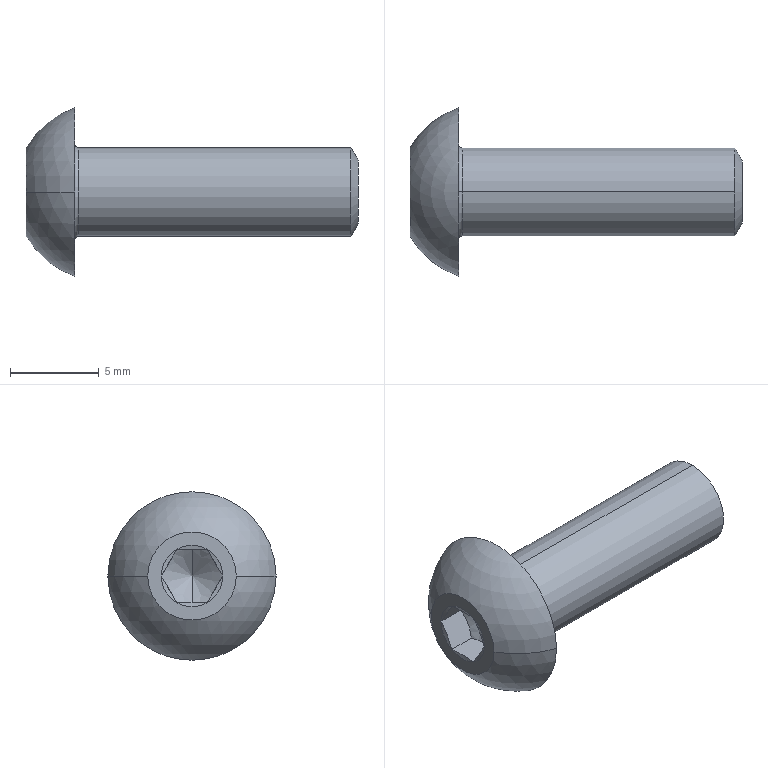Part | SolidWorks | features RevCut 2, Revolution 2, Cut 1, LPattern 1, RefAxis 1 | 1 solid | 25 faces | box 18.75 x 9.5 x 9.5 mm | volume 431.838 mm3 | cone 10 | plane 9 | torus 2 | sphere 2 | cylinder 2 | commonest cylinder face diameters 5 x2
STEP:
#1=CARTESIAN_POINT('',(0.,0.,1.807));
#2=VERTEX_POINT('',#1);
#3=CARTESIAN_POINT('',(0.,0.,-1.807));
#4=VERTEX_POINT('',#3);
#5=CARTESIAN_POINT('',(0.,0.,0.));
#6=DIRECTION('',(-1.,0.,0.));
#7=DIRECTION('',(0.,0.,1.));
#8=AXIS2_PLACEMENT_3D('',#5,#6,#7);
#9=CIRCLE('',#8,1.807);
#10=EDGE_CURVE('',#2,#4,#9,.T.);
#11=ORIENTED_EDGE('',*,*,#10,.T.);
#12=CARTESIAN_POINT('',(-0.4,0.,-2.5));
#13=VERTEX_POINT('',#12);
#14=CARTESIAN_POINT('',(-0.4,0.,-2.5));
#15=DIRECTION('',(-0.5,0.,-0.866));
#16=VECTOR('',#15,1000.);
#17=LINE('',#14,#16);
#18=EDGE_CURVE('',#4,#13,#17,.T.);
#19=ORIENTED_EDGE('',*,*,#18,.T.);
#20=CARTESIAN_POINT('',(-0.4,0.,2.5));
#21=VERTEX_POINT('',#20);
#22=CARTESIAN_POINT('',(-0.4,0.,0.));
#23=DIRECTION('',(-1.,0.,0.));
#24=DIRECTION('',(0.,0.,1.));
#25=AXIS2_PLACEMENT_3D('',#22,#23,#24);
#26=CIRCLE('',#25,2.5);
#27=EDGE_CURVE('',#21,#13,#26,.T.);
#28=ORIENTED_EDGE('',*,*,#27,.F.);
#29=CARTESIAN_POINT('',(-0.4,0.,2.5));
#30=DIRECTION('',(-0.5,0.,0.866));
#31=VECTOR('',#30,1000.);
#32=LINE('',#29,#31);
#33=EDGE_CURVE('',#2,#21,#32,.T.);
#34=ORIENTED_EDGE('',*,*,#33,.F.);
#35=EDGE_LOOP('',(#11,#19,#28,#34));
#36=FACE_OUTER_BOUND('',#35,.T.);
#37=CARTESIAN_POINT('',(-0.4,0.,0.));
#38=DIRECTION('',(-1.,0.,0.));
#39=DIRECTION('',(0.,0.,1.));
#40=AXIS2_PLACEMENT_3D('',#37,#38,#39);
#41=CONICAL_SURFACE('',#40,2.5,1.047);
#42=ADVANCED_FACE('',(#36),#41,.T.);
#43=CARTESIAN_POINT('',(-16.,0.,0.));
#44=VERTEX_POINT('',#43);
#45=CARTESIAN_POINT('',(-17.031,0.,1.5));
#46=VERTEX_POINT('',#45);
#47=CARTESIAN_POINT('',(-17.19,0.,1.732));
#48=DIRECTION('',(-0.5663,0.,0.8242));
#49=VECTOR('',#48,1000.);
#50=LINE('',#47,#49);
#51=EDGE_CURVE('',#44,#46,#50,.T.);
#52=ORIENTED_EDGE('',*,*,#51,.F.);
#53=CARTESIAN_POINT('',(-17.031,0.,-1.5));
#54=VERTEX_POINT('',#53);
#55=CARTESIAN_POINT('',(-17.19,0.,-1.732));
#56=DIRECTION('',(-0.5663,0.,-0.8242));
#57=VECTOR('',#56,1000.);
#58=LINE('',#55,#57);
#59=EDGE_CURVE('',#44,#54,#58,.T.);
#60=ORIENTED_EDGE('',*,*,#59,.T.);
#61=CARTESIAN_POINT('',(-17.19,-0.866,-1.5));
#62=VERTEX_POINT('',#61);
#63=CARTESIAN_POINT('',(-17.031,0.,-1.5));
#64=CARTESIAN_POINT('',(-17.031,-0.147,-1.5));
#65=CARTESIAN_POINT('',(-17.046,-0.2929,-1.5));
#66=CARTESIAN_POINT('',(-17.101,-0.5828,-1.5));
#67=CARTESIAN_POINT('',(-17.142,-0.7267,-1.5));
#68=CARTESIAN_POINT('',(-17.19,-0.866,-1.5));
#69=B_SPLINE_CURVE_WITH_KNOTS('',3,(#63,#64,#65,#66,#67,#68),.UNSPECIFIED.,.F.,.F.,(4,2,4),(0.005367,0.005808,0.006249),.UNSPECIFIED.);
#70=EDGE_CURVE('',#54,#62,#69,.T.);
#71=ORIENTED_EDGE('',*,*,#70,.T.);
#72=CARTESIAN_POINT('',(-17.19,-1.732,0.));
#73=VERTEX_POINT('',#72);
#74=CARTESIAN_POINT('',(-17.19,-0.866,-1.5));
#75=CARTESIAN_POINT('',(-17.094,-1.006,-1.257));
#76=CARTESIAN_POINT('',(-17.031,-1.149,-1.009));
#77=CARTESIAN_POINT('',(-17.03,-1.372,-0.6244));
#78=CARTESIAN_POINT('',(-17.046,-1.446,-0.4956));
#79=CARTESIAN_POINT('',(-17.102,-1.591,-0.2449));
#80=CARTESIAN_POINT('',(-17.142,-1.662,-0.1218));
#81=CARTESIAN_POINT('',(-17.19,-1.732,0.));
#82=B_SPLINE_CURVE_WITH_KNOTS('',3,(#74,#75,#76,#77,#78,#79,#80,#81),.UNSPECIFIED.,.F.,.F.,(4,2,2,4),(0.000000241,0.0008776,0.001316,0.001755),.UNSPECIFIED.);
#83=EDGE_CURVE('',#62,#73,#82,.T.);
#84=ORIENTED_EDGE('',*,*,#83,.T.);
#85=CARTESIAN_POINT('',(-17.19,-0.866,1.5));
#86=VERTEX_POINT('',#85);
#87=CARTESIAN_POINT('',(-17.19,-1.732,0.));
#88=CARTESIAN_POINT('',(-17.094,-1.592,0.2429));
#89=CARTESIAN_POINT('',(-17.031,-1.449,0.4906));
#90=CARTESIAN_POINT('',(-17.03,-1.227,0.8756));
#91=CARTESIAN_POINT('',(-17.046,-1.152,1.004));
#92=CARTESIAN_POINT('',(-17.102,-1.007,1.255));
#93=CARTESIAN_POINT('',(-17.142,-0.9363,1.378));
#94=CARTESIAN_POINT('',(-17.19,-0.866,1.5));
#95=B_SPLINE_CURVE_WITH_KNOTS('',3,(#87,#88,#89,#90,#91,#92,#93,#94),.UNSPECIFIED.,.F.,.F.,(4,2,2,4),(0.000000241,0.0008776,0.001316,0.001755),.UNSPECIFIED.);
#96=EDGE_CURVE('',#73,#86,#95,.T.);
#97=ORIENTED_EDGE('',*,*,#96,.T.);
#98=CARTESIAN_POINT('',(-17.19,-0.866,1.5));
#99=CARTESIAN_POINT('',(-17.142,-0.7267,1.5));
#100=CARTESIAN_POINT('',(-17.101,-0.5828,1.5));
#101=CARTESIAN_POINT('',(-17.046,-0.2929,1.5));
#102=CARTESIAN_POINT('',(-17.031,-0.147,1.5));
#103=CARTESIAN_POINT('',(-17.031,0.,1.5));
#104=B_SPLINE_CURVE_WITH_KNOTS('',3,(#98,#99,#100,#101,#102,#103),.UNSPECIFIED.,.F.,.F.,(4,2,4),(0.001244,0.001684,0.002125),.UNSPECIFIED.);
#105=EDGE_CURVE('',#86,#46,#104,.T.);
#106=ORIENTED_EDGE('',*,*,#105,.T.);
#107=EDGE_LOOP('',(#52,#60,#71,#84,#97,#106));
#108=FACE_OUTER_BOUND('',#107,.T.);
#109=CARTESIAN_POINT('',(-17.19,0.,0.));
#110=DIRECTION('',(-1.,0.,0.));
#111=DIRECTION('',(0.,0.,1.));
#112=AXIS2_PLACEMENT_3D('',#109,#110,#111);
#113=CONICAL_SURFACE('',#112,1.732,0.9688);
#114=ADVANCED_FACE('',(#108),#113,.F.);
#115=CARTESIAN_POINT('',(-16.,0.,-2.7));
#116=VERTEX_POINT('',#115);
#117=CARTESIAN_POINT('',(-16.,0.,2.7));
#118=VERTEX_POINT('',#117);
#119=CARTESIAN_POINT('',(-16.,0.,0.));
#120=DIRECTION('',(-1.,0.,0.));
#121=DIRECTION('',(0.,0.,1.));
#122=AXIS2_PLACEMENT_3D('',#119,#120,#121);
#123=CIRCLE('',#122,2.7);
#124=EDGE_CURVE('',#116,#118,#123,.T.);
#125=ORIENTED_EDGE('',*,*,#124,.F.);
#126=CARTESIAN_POINT('',(-15.8,0.,-2.5));
#127=VERTEX_POINT('',#126);
#128=CARTESIAN_POINT('',(-15.8,0.,-2.7));
#129=DIRECTION('',(0.,1.,0.));
#130=DIRECTION('',(0.,0.,1.));
#131=AXIS2_PLACEMENT_3D('',#128,#129,#130);
#132=CIRCLE('',#131,0.2);
#133=EDGE_CURVE('',#116,#127,#132,.T.);
#134=ORIENTED_EDGE('',*,*,#133,.T.);
#135=CARTESIAN_POINT('',(-15.8,0.,2.5));
#136=VERTEX_POINT('',#135);
#137=CARTESIAN_POINT('',(-15.8,0.,0.));
#138=DIRECTION('',(-1.,0.,0.));
#139=DIRECTION('',(0.,0.,1.));
#140=AXIS2_PLACEMENT_3D('',#137,#138,#139);
#141=CIRCLE('',#140,2.5);
#142=EDGE_CURVE('',#127,#136,#141,.T.);
#143=ORIENTED_EDGE('',*,*,#142,.T.);
#144=CARTESIAN_POINT('',(-15.8,0.,2.7));
#145=DIRECTION('',(0.,-1.,0.));
#146=DIRECTION('',(0.,0.,-1.));
#147=AXIS2_PLACEMENT_3D('',#144,#145,#146);
#148=CIRCLE('',#147,0.2);
#149=EDGE_CURVE('',#118,#136,#148,.T.);
#150=ORIENTED_EDGE('',*,*,#149,.F.);
#151=EDGE_LOOP('',(#125,#134,#143,#150));
#152=FACE_OUTER_BOUND('',#151,.T.);
#153=CARTESIAN_POINT('',(-15.8,0.,0.));
#154=DIRECTION('',(-1.,0.,0.));
#155=DIRECTION('',(0.,0.,1.));
#156=AXIS2_PLACEMENT_3D('',#153,#154,#155);
#157=TOROIDAL_SURFACE('',#156,2.7,0.2);
#158=ADVANCED_FACE('',(#152),#157,.F.);
#159=CARTESIAN_POINT('',(-16.,4.75,0.));
#160=VERTEX_POINT('',#159);
#161=CARTESIAN_POINT('',(-16.,-4.75,0.));
#162=VERTEX_POINT('',#161);
#163=CARTESIAN_POINT('',(-16.,0.,0.));
#164=DIRECTION('',(-1.,0.,0.));
#165=DIRECTION('',(0.,0.,1.));
#166=AXIS2_PLACEMENT_3D('',#163,#164,#165);
#167=CIRCLE('',#166,4.75);
#168=EDGE_CURVE('',#160,#162,#167,.T.);
#169=ORIENTED_EDGE('',*,*,#168,.T.);
#170=CARTESIAN_POINT('',(-18.75,-2.5,0.));
#171=VERTEX_POINT('',#170);
#172=CARTESIAN_POINT('',(-14.409,0.,0.));
#173=DIRECTION('',(0.,0.,-1.));
#174=DIRECTION('',(0.,1.,0.));
#175=AXIS2_PLACEMENT_3D('',#172,#173,#174);
#176=CIRCLE('',#175,5.009);
#177=EDGE_CURVE('',#162,#171,#176,.T.);
#178=ORIENTED_EDGE('',*,*,#177,.T.);
#179=CARTESIAN_POINT('',(-18.75,2.5,0.));
#180=VERTEX_POINT('',#179);
#181=CARTESIAN_POINT('',(-18.75,0.,0.));
#182=DIRECTION('',(-1.,0.,0.));
#183=DIRECTION('',(0.,0.,1.));
#184=AXIS2_PLACEMENT_3D('',#181,#182,#183);
#185=CIRCLE('',#184,2.5);
#186=EDGE_CURVE('',#180,#171,#185,.T.);
#187=ORIENTED_EDGE('',*,*,#186,.F.);
#188=CARTESIAN_POINT('',(-14.409,0.,0.));
#189=DIRECTION('',(0.,0.,1.));
#190=DIRECTION('',(1.,0.,0.));
#191=AXIS2_PLACEMENT_3D('',#188,#189,#190);
#192=CIRCLE('',#191,5.009);
#193=EDGE_CURVE('',#160,#180,#192,.T.);
#194=ORIENTED_EDGE('',*,*,#193,.F.);
#195=EDGE_LOOP('',(#169,#178,#187,#194));
#196=FACE_OUTER_BOUND('',#195,.T.);
#197=CARTESIAN_POINT('',(-14.409,0.,0.));
#198=DIRECTION('',(0.,0.,-1.));
#199=DIRECTION('',(0.,1.,0.));
#200=AXIS2_PLACEMENT_3D('',#197,#198,#199);
#201=SPHERICAL_SURFACE('',#200,5.009);
#202=ADVANCED_FACE('',(#196),#201,.T.);
#203=ORIENTED_EDGE('',*,*,#27,.T.);
#204=CARTESIAN_POINT('',(-18.75,0.,-2.5));
#205=DIRECTION('',(-1.,0.,0.));
#206=VECTOR('',#205,1000.);
#207=LINE('',#204,#206);
#208=EDGE_CURVE('',#13,#127,#207,.T.);
#209=ORIENTED_EDGE('',*,*,#208,.T.);
#210=CARTESIAN_POINT('',(-15.8,0.,0.));
#211=DIRECTION('',(-1.,0.,0.));
#212=DIRECTION('',(0.,0.,1.));
#213=AXIS2_PLACEMENT_3D('',#210,#211,#212);
#214=CIRCLE('',#213,2.5);
#215=EDGE_CURVE('',#136,#127,#214,.T.);
#216=ORIENTED_EDGE('',*,*,#215,.F.);
#217=CARTESIAN_POINT('',(-18.75,0.,2.5));
#218=DIRECTION('',(-1.,0.,0.));
#219=VECTOR('',#218,1000.);
#220=LINE('',#217,#219);
#221=EDGE_CURVE('',#21,#136,#220,.T.);
#222=ORIENTED_EDGE('',*,*,#221,.F.);
#223=EDGE_LOOP('',(#203,#209,#216,#222));
#224=FACE_OUTER_BOUND('',#223,.T.);
#225=CARTESIAN_POINT('',(-18.75,0.,0.));
#226=DIRECTION('',(-1.,0.,0.));
#227=DIRECTION('',(0.,0.,1.));
#228=AXIS2_PLACEMENT_3D('',#225,#226,#227);
#229=CYLINDRICAL_SURFACE('',#228,2.5);
#230=ADVANCED_FACE('',(#224),#229,.T.);
#231=ORIENTED_EDGE('',*,*,#208,.F.);
#232=CARTESIAN_POINT('',(-0.4,0.,0.));
#233=DIRECTION('',(-1.,0.,0.));
#234=DIRECTION('',(0.,0.,1.));
#235=AXIS2_PLACEMENT_3D('',#232,#233,#234);
#236=CIRCLE('',#235,2.5);
#237=EDGE_CURVE('',#13,#21,#236,.T.);
#238=ORIENTED_EDGE('',*,*,#237,.T.);
#239=ORIENTED_EDGE('',*,*,#221,.T.);
#240=ORIENTED_EDGE('',*,*,#142,.F.);
#241=EDGE_LOOP('',(#231,#238,#239,#240));
#242=FACE_OUTER_BOUND('',#241,.T.);
#243=CARTESIAN_POINT('',(-18.75,0.,0.));
#244=DIRECTION('',(-1.,0.,0.));
#245=DIRECTION('',(0.,0.,1.));
#246=AXIS2_PLACEMENT_3D('',#243,#244,#245);
#247=CYLINDRICAL_SURFACE('',#246,2.5);
#248=ADVANCED_FACE('',(#242),#247,.T.);
#249=ORIENTED_EDGE('',*,*,#186,.T.);
#250=CARTESIAN_POINT('',(-18.75,0.,0.));
#251=DIRECTION('',(-1.,0.,0.));
#252=DIRECTION('',(0.,0.,1.));
#253=AXIS2_PLACEMENT_3D('',#250,#251,#252);
#254=CIRCLE('',#253,2.5);
#255=EDGE_CURVE('',#171,#180,#254,.T.);
#256=ORIENTED_EDGE('',*,*,#255,.T.);
#257=EDGE_LOOP('',(#249,#256));
#258=FACE_OUTER_BOUND('',#257,.T.);
#259=CARTESIAN_POINT('',(-18.75,-0.866,-1.5));
#260=VERTEX_POINT('',#259);
#261=CARTESIAN_POINT('',(-18.75,-1.732,0.));
#262=VERTEX_POINT('',#261);
#263=CARTESIAN_POINT('',(-18.75,0.,0.));
#264=DIRECTION('',(-1.,0.,0.));
#265=DIRECTION('',(0.,0.,-1.));
#266=AXIS2_PLACEMENT_3D('',#263,#264,#265);
#267=CIRCLE('',#266,1.732);
#268=EDGE_CURVE('',#260,#262,#267,.T.);
#269=ORIENTED_EDGE('',*,*,#268,.F.);
#270=CARTESIAN_POINT('',(-18.75,0.866,-1.5));
#271=VERTEX_POINT('',#270);
#272=CARTESIAN_POINT('',(-18.75,0.,0.));
#273=DIRECTION('',(-1.,0.,0.));
#274=DIRECTION('',(0.,0.,-1.));
#275=AXIS2_PLACEMENT_3D('',#272,#273,#274);
#276=CIRCLE('',#275,1.732);
#277=EDGE_CURVE('',#271,#260,#276,.T.);
#278=ORIENTED_EDGE('',*,*,#277,.F.);
#279=CARTESIAN_POINT('',(-18.75,1.732,0.));
#280=VERTEX_POINT('',#279);
#281=CARTESIAN_POINT('',(-18.75,0.,0.));
#282=DIRECTION('',(-1.,0.,0.));
#283=DIRECTION('',(0.,0.,-1.));
#284=AXIS2_PLACEMENT_3D('',#281,#282,#283);
#285=CIRCLE('',#284,1.732);
#286=EDGE_CURVE('',#280,#271,#285,.T.);
#287=ORIENTED_EDGE('',*,*,#286,.F.);
#288=CARTESIAN_POINT('',(-18.75,0.866,1.5));
#289=VERTEX_POINT('',#288);
#290=CARTESIAN_POINT('',(-18.75,0.,0.));
#291=DIRECTION('',(-1.,0.,0.));
#292=DIRECTION('',(0.,0.,-1.));
#293=AXIS2_PLACEMENT_3D('',#290,#291,#292);
#294=CIRCLE('',#293,1.732);
#295=EDGE_CURVE('',#289,#280,#294,.T.);
#296=ORIENTED_EDGE('',*,*,#295,.F.);
#297=CARTESIAN_POINT('',(-18.75,-0.866,1.5));
#298=VERTEX_POINT('',#297);
#299=CARTESIAN_POINT('',(-18.75,0.,0.));
#300=DIRECTION('',(-1.,0.,0.));
#301=DIRECTION('',(0.,0.,-1.));
#302=AXIS2_PLACEMENT_3D('',#299,#300,#301);
#303=CIRCLE('',#302,1.732);
#304=EDGE_CURVE('',#298,#289,#303,.T.);
#305=ORIENTED_EDGE('',*,*,#304,.F.);
#306=CARTESIAN_POINT('',(-18.75,0.,0.));
#307=DIRECTION('',(-1.,0.,0.));
#308=DIRECTION('',(0.,-1.,0.));
#309=AXIS2_PLACEMENT_3D('',#306,#307,#308);
#310=CIRCLE('',#309,1.732);
#311=EDGE_CURVE('',#262,#298,#310,.T.);
#312=ORIENTED_EDGE('',*,*,#311,.F.);
#313=EDGE_LOOP('',(#269,#278,#287,#296,#305,#312));
#314=FACE_BOUND('',#313,.T.);
#315=CARTESIAN_POINT('',(-18.75,0.,0.));
#316=DIRECTION('',(1.,0.,0.));
#317=DIRECTION('',(0.,0.,-1.));
#318=AXIS2_PLACEMENT_3D('',#315,#316,#317);
#319=PLANE('',#318);
#320=ADVANCED_FACE('',(#258,#314),#319,.F.);
#321=ORIENTED_EDGE('',*,*,#177,.F.);
#322=CARTESIAN_POINT('',(-16.,0.,0.));
#323=DIRECTION('',(-1.,0.,0.));
#324=DIRECTION('',(0.,0.,1.));
#325=AXIS2_PLACEMENT_3D('',#322,#323,#324);
#326=CIRCLE('',#325,4.75);
#327=EDGE_CURVE('',#162,#160,#326,.T.);
#328=ORIENTED_EDGE('',*,*,#327,.T.);
#329=ORIENTED_EDGE('',*,*,#193,.T.);
#330=ORIENTED_EDGE('',*,*,#255,.F.);
#331=EDGE_LOOP('',(#321,#328,#329,#330));
#332=FACE_OUTER_BOUND('',#331,.T.);
#333=CARTESIAN_POINT('',(-14.409,0.,0.));
#334=DIRECTION('',(0.,0.,-1.));
#335=DIRECTION('',(0.,1.,0.));
#336=AXIS2_PLACEMENT_3D('',#333,#334,#335);
#337=SPHERICAL_SURFACE('',#336,5.009);
#338=ADVANCED_FACE('',(#332),#337,.T.);
#339=ORIENTED_EDGE('',*,*,#168,.F.);
#340=ORIENTED_EDGE('',*,*,#327,.F.);
#341=EDGE_LOOP('',(#339,#340));
#342=FACE_OUTER_BOUND('',#341,.T.);
#343=CARTESIAN_POINT('',(-16.,0.,0.));
#344=DIRECTION('',(-1.,0.,0.));
#345=DIRECTION('',(0.,0.,1.));
#346=AXIS2_PLACEMENT_3D('',#343,#344,#345);
#347=CIRCLE('',#346,2.7);
#348=EDGE_CURVE('',#118,#116,#347,.T.);
#349=ORIENTED_EDGE('',*,*,#348,.T.);
#350=ORIENTED_EDGE('',*,*,#124,.T.);
#351=EDGE_LOOP('',(#349,#350));
#352=FACE_BOUND('',#351,.T.);
#353=CARTESIAN_POINT('',(-16.,2.7,0.));
#354=DIRECTION('',(-1.,0.,0.));
#355=DIRECTION('',(0.,0.,1.));
#356=AXIS2_PLACEMENT_3D('',#353,#354,#355);
#357=PLANE('',#356);
#358=ADVANCED_FACE('',(#342,#352),#357,.F.);
#359=ORIENTED_EDGE('',*,*,#133,.F.);
#360=ORIENTED_EDGE('',*,*,#348,.F.);
#361=ORIENTED_EDGE('',*,*,#149,.T.);
#362=ORIENTED_EDGE('',*,*,#215,.T.);
#363=EDGE_LOOP('',(#359,#360,#361,#362));
#364=FACE_OUTER_BOUND('',#363,.T.);
#365=CARTESIAN_POINT('',(-15.8,0.,0.));
#366=DIRECTION('',(-1.,0.,0.));
#367=DIRECTION('',(0.,0.,1.));
#368=AXIS2_PLACEMENT_3D('',#365,#366,#367);
#369=TOROIDAL_SURFACE('',#368,2.7,0.2);
#370=ADVANCED_FACE('',(#364),#369,.F.);
#371=CARTESIAN_POINT('',(-18.75,-0.866,-1.5));
#372=CARTESIAN_POINT('',(-18.713,-0.5778,-1.5));
#373=CARTESIAN_POINT('',(-18.691,-0.2874,-1.5));
#374=CARTESIAN_POINT('',(-18.691,0.2902,-1.5));
#375=CARTESIAN_POINT('',(-18.713,0.5783,-1.5));
#376=CARTESIAN_POINT('',(-18.75,0.866,-1.5));
#377=B_SPLINE_CURVE_WITH_KNOTS('',3,(#371,#372,#373,#374,#375,#376),.UNSPECIFIED.,.F.,.F.,(4,2,4),(0.001419,0.00229,0.003161),.UNSPECIFIED.);
#378=EDGE_CURVE('',#260,#271,#377,.T.);
#379=ORIENTED_EDGE('',*,*,#378,.T.);
#380=ORIENTED_EDGE('',*,*,#277,.T.);
#381=EDGE_LOOP('',(#379,#380));
#382=FACE_OUTER_BOUND('',#381,.T.);
#383=CARTESIAN_POINT('',(-1018.31,0.,0.));
#384=DIRECTION('',(-1.,0.,0.));
#385=DIRECTION('',(0.,-1.,0.));
#386=AXIS2_PLACEMENT_3D('',#383,#384,#385);
#387=CONICAL_SURFACE('',#386,3936.479,1.322);
#388=ADVANCED_FACE('',(#382),#387,.F.);
#389=CARTESIAN_POINT('',(-18.75,0.866,-1.5));
#390=CARTESIAN_POINT('',(-18.713,1.01,-1.25));
#391=CARTESIAN_POINT('',(-18.669,1.299,-0.75));
#392=CARTESIAN_POINT('',(-18.713,1.588,-0.25));
#393=CARTESIAN_POINT('',(-18.75,1.732,0.));
#394=B_SPLINE_CURVE_WITH_KNOTS('',3,(#389,#390,#391,#392,#393),.UNSPECIFIED.,.F.,.F.,(4,1,4),(0.000000231,0.0008663,0.001732),.UNSPECIFIED.);
#395=EDGE_CURVE('',#271,#280,#394,.T.);
#396=ORIENTED_EDGE('',*,*,#395,.T.);
#397=ORIENTED_EDGE('',*,*,#286,.T.);
#398=EDGE_LOOP('',(#396,#397));
#399=FACE_OUTER_BOUND('',#398,.T.);
#400=CARTESIAN_POINT('',(-1018.31,0.,0.));
#401=DIRECTION('',(-1.,0.,0.));
#402=DIRECTION('',(0.,-1.,0.));
#403=AXIS2_PLACEMENT_3D('',#400,#401,#402);
#404=CONICAL_SURFACE('',#403,3936.479,1.322);
#405=ADVANCED_FACE('',(#399),#404,.F.);
#406=CARTESIAN_POINT('',(-18.75,1.732,0.));
#407=CARTESIAN_POINT('',(-18.713,1.588,0.25));
#408=CARTESIAN_POINT('',(-18.669,1.299,0.75));
#409=CARTESIAN_POINT('',(-18.713,1.01,1.25));
#410=CARTESIAN_POINT('',(-18.75,0.866,1.5));
#411=B_SPLINE_CURVE_WITH_KNOTS('',3,(#406,#407,#408,#409,#410),.UNSPECIFIED.,.F.,.F.,(4,1,4),(0.000000231,0.0008663,0.001732),.UNSPECIFIED.);
#412=EDGE_CURVE('',#280,#289,#411,.T.);
#413=ORIENTED_EDGE('',*,*,#412,.T.);
#414=ORIENTED_EDGE('',*,*,#295,.T.);
#415=EDGE_LOOP('',(#413,#414));
#416=FACE_OUTER_BOUND('',#415,.T.);
#417=CARTESIAN_POINT('',(-1018.31,0.,0.));
#418=DIRECTION('',(-1.,0.,0.));
#419=DIRECTION('',(0.,-1.,0.));
#420=AXIS2_PLACEMENT_3D('',#417,#418,#419);
#421=CONICAL_SURFACE('',#420,3936.479,1.322);
#422=ADVANCED_FACE('',(#416),#421,.F.);
#423=CARTESIAN_POINT('',(-18.75,0.866,1.5));
#424=CARTESIAN_POINT('',(-18.713,0.5783,1.5));
#425=CARTESIAN_POINT('',(-18.691,0.2902,1.5));
#426=CARTESIAN_POINT('',(-18.691,-0.2874,1.5));
#427=CARTESIAN_POINT('',(-18.713,-0.5778,1.5));
#428=CARTESIAN_POINT('',(-18.75,-0.866,1.5));
#429=B_SPLINE_CURVE_WITH_KNOTS('',3,(#423,#424,#425,#426,#427,#428),.UNSPECIFIED.,.F.,.F.,(4,2,4),(0.003564,0.004433,0.005303),.UNSPECIFIED.);
#430=EDGE_CURVE('',#289,#298,#429,.T.);
#431=ORIENTED_EDGE('',*,*,#430,.T.);
#432=ORIENTED_EDGE('',*,*,#304,.T.);
#433=EDGE_LOOP('',(#431,#432));
#434=FACE_OUTER_BOUND('',#433,.T.);
#435=CARTESIAN_POINT('',(-1018.31,0.,0.));
#436=DIRECTION('',(-1.,0.,0.));
#437=DIRECTION('',(0.,-1.,0.));
#438=AXIS2_PLACEMENT_3D('',#435,#436,#437);
#439=CONICAL_SURFACE('',#438,3936.479,1.322);
#440=ADVANCED_FACE('',(#434),#439,.F.);
#441=CARTESIAN_POINT('',(-18.75,-0.866,1.5));
#442=CARTESIAN_POINT('',(-18.713,-1.01,1.25));
#443=CARTESIAN_POINT('',(-18.669,-1.299,0.75));
#444=CARTESIAN_POINT('',(-18.713,-1.588,0.25));
#445=CARTESIAN_POINT('',(-18.75,-1.732,0.));
#446=B_SPLINE_CURVE_WITH_KNOTS('',3,(#441,#442,#443,#444,#445),.UNSPECIFIED.,.F.,.F.,(4,1,4),(0.000000231,0.0008663,0.001732),.UNSPECIFIED.);
#447=EDGE_CURVE('',#298,#262,#446,.T.);
#448=ORIENTED_EDGE('',*,*,#447,.T.);
#449=ORIENTED_EDGE('',*,*,#311,.T.);
#450=EDGE_LOOP('',(#448,#449));
#451=FACE_OUTER_BOUND('',#450,.T.);
#452=CARTESIAN_POINT('',(-1018.31,0.,0.));
#453=DIRECTION('',(-1.,0.,0.));
#454=DIRECTION('',(0.,-1.,0.));
#455=AXIS2_PLACEMENT_3D('',#452,#453,#454);
#456=CONICAL_SURFACE('',#455,3936.479,1.322);
#457=ADVANCED_FACE('',(#451),#456,.F.);
#458=CARTESIAN_POINT('',(-18.75,-1.732,0.));
#459=CARTESIAN_POINT('',(-18.713,-1.588,-0.25));
#460=CARTESIAN_POINT('',(-18.669,-1.299,-0.75));
#461=CARTESIAN_POINT('',(-18.713,-1.01,-1.25));
#462=CARTESIAN_POINT('',(-18.75,-0.866,-1.5));
#463=B_SPLINE_CURVE_WITH_KNOTS('',3,(#458,#459,#460,#461,#462),.UNSPECIFIED.,.F.,.F.,(4,1,4),(0.000000231,0.0008663,0.001732),.UNSPECIFIED.);
#464=EDGE_CURVE('',#262,#260,#463,.T.);
#465=ORIENTED_EDGE('',*,*,#464,.T.);
#466=ORIENTED_EDGE('',*,*,#268,.T.);
#467=EDGE_LOOP('',(#465,#466));
#468=FACE_OUTER_BOUND('',#467,.T.);
#469=CARTESIAN_POINT('',(-1018.31,0.,0.));
#470=DIRECTION('',(-1.,0.,0.));
#471=DIRECTION('',(0.,-1.,0.));
#472=AXIS2_PLACEMENT_3D('',#469,#470,#471);
#473=CONICAL_SURFACE('',#472,3936.479,1.322);
#474=ADVANCED_FACE('',(#468),#473,.F.);
#475=ORIENTED_EDGE('',*,*,#59,.F.);
#476=ORIENTED_EDGE('',*,*,#51,.T.);
#477=CARTESIAN_POINT('',(-17.19,0.866,1.5));
#478=VERTEX_POINT('',#477);
#479=CARTESIAN_POINT('',(-17.031,0.,1.5));
#480=CARTESIAN_POINT('',(-17.031,0.1469,1.5));
#481=CARTESIAN_POINT('',(-17.046,0.2963,1.5));
#482=CARTESIAN_POINT('',(-17.102,0.5859,1.5));
#483=CARTESIAN_POINT('',(-17.142,0.7271,1.5));
#484=CARTESIAN_POINT('',(-17.19,0.866,1.5));
#485=B_SPLINE_CURVE_WITH_KNOTS('',3,(#479,#480,#481,#482,#483,#484),.UNSPECIFIED.,.F.,.F.,(4,2,4),(0.002125,0.002565,0.003005),.UNSPECIFIED.);
#486=EDGE_CURVE('',#46,#478,#485,.T.);
#487=ORIENTED_EDGE('',*,*,#486,.T.);
#488=CARTESIAN_POINT('',(-17.19,1.732,0.));
#489=VERTEX_POINT('',#488);
#490=CARTESIAN_POINT('',(-17.19,0.866,1.5));
#491=CARTESIAN_POINT('',(-17.094,1.006,1.257));
#492=CARTESIAN_POINT('',(-17.031,1.149,1.009));
#493=CARTESIAN_POINT('',(-17.03,1.372,0.6244));
#494=CARTESIAN_POINT('',(-17.046,1.446,0.4956));
#495=CARTESIAN_POINT('',(-17.102,1.591,0.2449));
#496=CARTESIAN_POINT('',(-17.142,1.662,0.1218));
#497=CARTESIAN_POINT('',(-17.19,1.732,0.));
#498=B_SPLINE_CURVE_WITH_KNOTS('',3,(#490,#491,#492,#493,#494,#495,#496,#497),.UNSPECIFIED.,.F.,.F.,(4,2,2,4),(0.000000241,0.0008776,0.001316,0.001755),.UNSPECIFIED.);
#499=EDGE_CURVE('',#478,#489,#498,.T.);
#500=ORIENTED_EDGE('',*,*,#499,.T.);
#501=CARTESIAN_POINT('',(-17.19,0.866,-1.5));
#502=VERTEX_POINT('',#501);
#503=CARTESIAN_POINT('',(-17.19,1.732,0.));
#504=CARTESIAN_POINT('',(-17.094,1.592,-0.2429));
#505=CARTESIAN_POINT('',(-17.031,1.449,-0.4906));
#506=CARTESIAN_POINT('',(-17.03,1.227,-0.8756));
#507=CARTESIAN_POINT('',(-17.046,1.152,-1.004));
#508=CARTESIAN_POINT('',(-17.102,1.007,-1.255));
#509=CARTESIAN_POINT('',(-17.142,0.9363,-1.378));
#510=CARTESIAN_POINT('',(-17.19,0.866,-1.5));
#511=B_SPLINE_CURVE_WITH_KNOTS('',3,(#503,#504,#505,#506,#507,#508,#509,#510),.UNSPECIFIED.,.F.,.F.,(4,2,2,4),(0.000000241,0.0008776,0.001316,0.001755),.UNSPECIFIED.);
#512=EDGE_CURVE('',#489,#502,#511,.T.);
#513=ORIENTED_EDGE('',*,*,#512,.T.);
#514=CARTESIAN_POINT('',(-17.19,0.866,-1.5));
#515=CARTESIAN_POINT('',(-17.142,0.7271,-1.5));
#516=CARTESIAN_POINT('',(-17.102,0.5859,-1.5));
#517=CARTESIAN_POINT('',(-17.046,0.2963,-1.5));
#518=CARTESIAN_POINT('',(-17.031,0.1469,-1.5));
#519=CARTESIAN_POINT('',(-17.031,0.,-1.5));
#520=B_SPLINE_CURVE_WITH_KNOTS('',3,(#514,#515,#516,#517,#518,#519),.UNSPECIFIED.,.F.,.F.,(4,2,4),(0.004486,0.004926,0.005367),.UNSPECIFIED.);
#521=EDGE_CURVE('',#502,#54,#520,.T.);
#522=ORIENTED_EDGE('',*,*,#521,.T.);
#523=EDGE_LOOP('',(#475,#476,#487,#500,#513,#522));
#524=FACE_OUTER_BOUND('',#523,.T.);
#525=CARTESIAN_POINT('',(-17.19,0.,0.));
#526=DIRECTION('',(-1.,0.,0.));
#527=DIRECTION('',(0.,0.,1.));
#528=AXIS2_PLACEMENT_3D('',#525,#526,#527);
#529=CONICAL_SURFACE('',#528,1.732,0.9688);
#530=ADVANCED_FACE('',(#524),#529,.F.);
#531=ORIENTED_EDGE('',*,*,#395,.F.);
#532=CARTESIAN_POINT('',(-16.,0.866,-1.5));
#533=DIRECTION('',(-1.,0.,0.));
#534=VECTOR('',#533,1000.);
#535=LINE('',#532,#534);
#536=EDGE_CURVE('',#502,#271,#535,.T.);
#537=ORIENTED_EDGE('',*,*,#536,.F.);
#538=ORIENTED_EDGE('',*,*,#512,.F.);
#539=CARTESIAN_POINT('',(-16.,1.732,0.));
#540=DIRECTION('',(-1.,0.,0.));
#541=VECTOR('',#540,1000.);
#542=LINE('',#539,#541);
#543=EDGE_CURVE('',#489,#280,#542,.T.);
#544=ORIENTED_EDGE('',*,*,#543,.T.);
#545=EDGE_LOOP('',(#531,#537,#538,#544));
#546=FACE_OUTER_BOUND('',#545,.T.);
#547=CARTESIAN_POINT('',(-16.,1.732,0.));
#548=DIRECTION('',(0.,0.866,-0.5));
#549=DIRECTION('',(0.,0.5,0.866));
#550=AXIS2_PLACEMENT_3D('',#547,#548,#549);
#551=PLANE('',#550);
#552=ADVANCED_FACE('',(#546),#551,.F.);
#553=ORIENTED_EDGE('',*,*,#378,.F.);
#554=CARTESIAN_POINT('',(-16.,-0.866,-1.5));
#555=DIRECTION('',(-1.,0.,0.));
#556=VECTOR('',#555,1000.);
#557=LINE('',#554,#556);
#558=EDGE_CURVE('',#62,#260,#557,.T.);
#559=ORIENTED_EDGE('',*,*,#558,.F.);
#560=ORIENTED_EDGE('',*,*,#70,.F.);
#561=ORIENTED_EDGE('',*,*,#521,.F.);
#562=ORIENTED_EDGE('',*,*,#536,.T.);
#563=EDGE_LOOP('',(#553,#559,#560,#561,#562));
#564=FACE_OUTER_BOUND('',#563,.T.);
#565=CARTESIAN_POINT('',(-16.,0.866,-1.5));
#566=DIRECTION('',(0.,0.,-1.));
#567=DIRECTION('',(-1.,0.,0.));
#568=AXIS2_PLACEMENT_3D('',#565,#566,#567);
#569=PLANE('',#568);
#570=ADVANCED_FACE('',(#564),#569,.F.);
#571=ORIENTED_EDGE('',*,*,#464,.F.);
#572=CARTESIAN_POINT('',(-16.,-1.732,0.));
#573=DIRECTION('',(-1.,0.,0.));
#574=VECTOR('',#573,1000.);
#575=LINE('',#572,#574);
#576=EDGE_CURVE('',#73,#262,#575,.T.);
#577=ORIENTED_EDGE('',*,*,#576,.F.);
#578=ORIENTED_EDGE('',*,*,#83,.F.);
#579=ORIENTED_EDGE('',*,*,#558,.T.);
#580=EDGE_LOOP('',(#571,#577,#578,#579));
#581=FACE_OUTER_BOUND('',#580,.T.);
#582=CARTESIAN_POINT('',(-16.,-0.866,-1.5));
#583=DIRECTION('',(0.,-0.866,-0.5));
#584=DIRECTION('',(0.,0.5,-0.866));
#585=AXIS2_PLACEMENT_3D('',#582,#583,#584);
#586=PLANE('',#585);
#587=ADVANCED_FACE('',(#581),#586,.F.);
#588=ORIENTED_EDGE('',*,*,#447,.F.);
#589=CARTESIAN_POINT('',(-16.,-0.866,1.5));
#590=DIRECTION('',(-1.,0.,0.));
#591=VECTOR('',#590,1000.);
#592=LINE('',#589,#591);
#593=EDGE_CURVE('',#86,#298,#592,.T.);
#594=ORIENTED_EDGE('',*,*,#593,.F.);
#595=ORIENTED_EDGE('',*,*,#96,.F.);
#596=ORIENTED_EDGE('',*,*,#576,.T.);
#597=EDGE_LOOP('',(#588,#594,#595,#596));
#598=FACE_OUTER_BOUND('',#597,.T.);
#599=CARTESIAN_POINT('',(-16.,-1.732,0.));
#600=DIRECTION('',(0.,-0.866,0.5));
#601=DIRECTION('',(0.,-0.5,-0.866));
#602=AXIS2_PLACEMENT_3D('',#599,#600,#601);
#603=PLANE('',#602);
#604=ADVANCED_FACE('',(#598),#603,.F.);
#605=ORIENTED_EDGE('',*,*,#430,.F.);
#606=CARTESIAN_POINT('',(-16.,0.866,1.5));
#607=DIRECTION('',(-1.,0.,0.));
#608=VECTOR('',#607,1000.);
#609=LINE('',#606,#608);
#610=EDGE_CURVE('',#478,#289,#609,.T.);
#611=ORIENTED_EDGE('',*,*,#610,.F.);
#612=ORIENTED_EDGE('',*,*,#486,.F.);
#613=ORIENTED_EDGE('',*,*,#105,.F.);
#614=ORIENTED_EDGE('',*,*,#593,.T.);
#615=EDGE_LOOP('',(#605,#611,#612,#613,#614));
#616=FACE_OUTER_BOUND('',#615,.T.);
#617=CARTESIAN_POINT('',(-16.,-0.866,1.5));
#618=DIRECTION('',(0.,0.,1.));
#619=DIRECTION('',(0.,-1.,0.));
#620=AXIS2_PLACEMENT_3D('',#617,#618,#619);
#621=PLANE('',#620);
#622=ADVANCED_FACE('',(#616),#621,.F.);
#623=ORIENTED_EDGE('',*,*,#412,.F.);
#624=ORIENTED_EDGE('',*,*,#543,.F.);
#625=ORIENTED_EDGE('',*,*,#499,.F.);
#626=ORIENTED_EDGE('',*,*,#610,.T.);
#627=EDGE_LOOP('',(#623,#624,#625,#626));
#628=FACE_OUTER_BOUND('',#627,.T.);
#629=CARTESIAN_POINT('',(-16.,0.866,1.5));
#630=DIRECTION('',(0.,0.866,0.5));
#631=DIRECTION('',(0.,-0.5,0.866));
#632=AXIS2_PLACEMENT_3D('',#629,#630,#631);
#633=PLANE('',#632);
#634=ADVANCED_FACE('',(#628),#633,.F.);
#635=ORIENTED_EDGE('',*,*,#18,.F.);
#636=CARTESIAN_POINT('',(0.,0.,0.));
#637=DIRECTION('',(-1.,0.,0.));
#638=DIRECTION('',(0.,0.,1.));
#639=AXIS2_PLACEMENT_3D('',#636,#637,#638);
#640=CIRCLE('',#639,1.807);
#641=EDGE_CURVE('',#4,#2,#640,.T.);
#642=ORIENTED_EDGE('',*,*,#641,.T.);
#643=ORIENTED_EDGE('',*,*,#33,.T.);
#644=ORIENTED_EDGE('',*,*,#237,.F.);
#645=EDGE_LOOP('',(#635,#642,#643,#644));
#646=FACE_OUTER_BOUND('',#645,.T.);
#647=CARTESIAN_POINT('',(-0.4,0.,0.));
#648=DIRECTION('',(-1.,0.,0.));
#649=DIRECTION('',(0.,0.,1.));
#650=AXIS2_PLACEMENT_3D('',#647,#648,#649);
#651=CONICAL_SURFACE('',#650,2.5,1.047);
#652=ADVANCED_FACE('',(#646),#651,.T.);
#653=ORIENTED_EDGE('',*,*,#10,.F.);
#654=ORIENTED_EDGE('',*,*,#641,.F.);
#655=EDGE_LOOP('',(#653,#654));
#656=FACE_OUTER_BOUND('',#655,.T.);
#657=CARTESIAN_POINT('',(0.,2.5,0.));
#658=DIRECTION('',(-1.,0.,0.));
#659=DIRECTION('',(0.,0.,1.));
#660=AXIS2_PLACEMENT_3D('',#657,#658,#659);
#661=PLANE('',#660);
#662=ADVANCED_FACE('',(#656),#661,.F.);
#663=CLOSED_SHELL('',(#42,#114,#158,#202,#230,#248,#320,#338,#358,#370,#388,#405,#422,#440,#457,#474,#530,#552,#570,#587,#604,#622,#634,#652,#662));
#664=MANIFOLD_SOLID_BREP('',#663);
#665=CARTESIAN_POINT('',(0.,0.,0.));
#666=DIRECTION('',(0.,0.,1.));
#667=DIRECTION('',(1.,0.,0.));
#668=AXIS2_PLACEMENT_3D('',#665,#666,#667);
#669=(LENGTH_UNIT()NAMED_UNIT(*)SI_UNIT(.MILLI.,.METRE.));
#670=UNCERTAINTY_MEASURE_WITH_UNIT(LENGTH_MEASURE(0.00001),#669,'','');
#671=(NAMED_UNIT(*)PLANE_ANGLE_UNIT()SI_UNIT($,.RADIAN.));
#672=(NAMED_UNIT(*)SI_UNIT($,.STERADIAN.)SOLID_ANGLE_UNIT());
#673=(GEOMETRIC_REPRESENTATION_CONTEXT(3)GLOBAL_UNCERTAINTY_ASSIGNED_CONTEXT((#670))GLOBAL_UNIT_ASSIGNED_CONTEXT((#669,#671,#672))REPRESENTATION_CONTEXT('',''));
#674=ADVANCED_BREP_SHAPE_REPRESENTATION('',(#664,#668),#673);